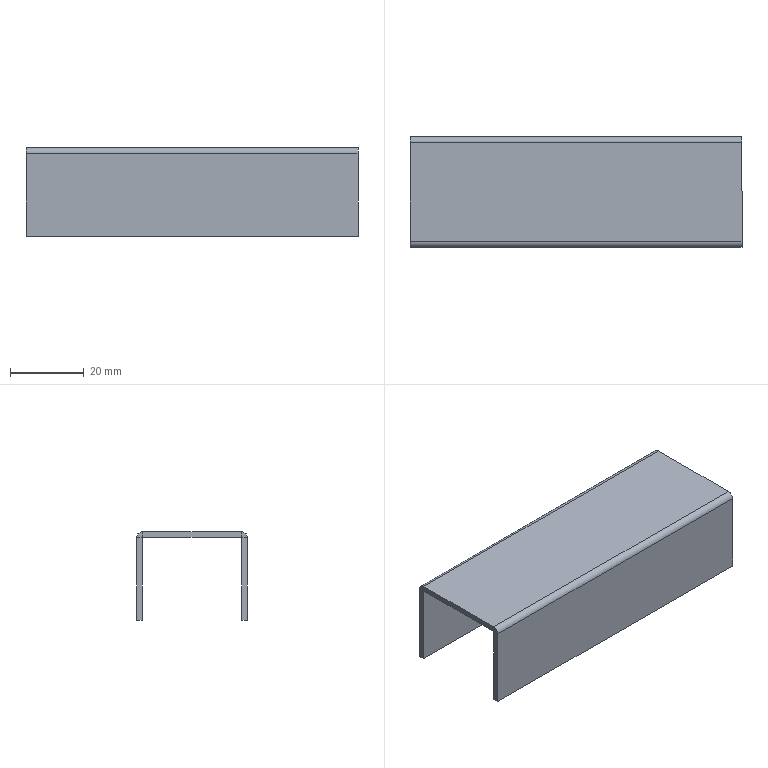Part | SolidWorks | features EdgeFlange 1, FlatPattern 1, SMBaseFlange 1, SheetMetal 1 | 1 solid | 22 faces | box 90 x 30 x 24 mm | volume 10026 mm3 | plane 18 | cylinder 4 | commonest cylinder face diameters 0.2 x2 3.2 x2
STEP:
#1=CARTESIAN_POINT('',(-45.,-13.4,-1.5));
#2=VERTEX_POINT('',#1);
#3=CARTESIAN_POINT('',(45.,-13.4,-1.5));
#4=VERTEX_POINT('',#3);
#5=CARTESIAN_POINT('',(-45.,-13.4,-1.5));
#6=DIRECTION('',(1.,0.,0.));
#7=VECTOR('',#6,1000.);
#8=LINE('',#5,#7);
#9=EDGE_CURVE('',#2,#4,#8,.T.);
#10=ORIENTED_EDGE('',*,*,#9,.F.);
#11=CARTESIAN_POINT('',(-45.,13.4,-1.5));
#12=VERTEX_POINT('',#11);
#13=CARTESIAN_POINT('',(-45.,15.,-1.5));
#14=DIRECTION('',(0.,-1.,0.));
#15=VECTOR('',#14,1000.);
#16=LINE('',#13,#15);
#17=EDGE_CURVE('',#12,#2,#16,.T.);
#18=ORIENTED_EDGE('',*,*,#17,.F.);
#19=CARTESIAN_POINT('',(45.,13.4,-1.5));
#20=VERTEX_POINT('',#19);
#21=CARTESIAN_POINT('',(45.,13.4,-1.5));
#22=DIRECTION('',(-1.,0.,0.));
#23=VECTOR('',#22,1000.);
#24=LINE('',#21,#23);
#25=EDGE_CURVE('',#20,#12,#24,.T.);
#26=ORIENTED_EDGE('',*,*,#25,.F.);
#27=CARTESIAN_POINT('',(45.,15.,-1.5));
#28=DIRECTION('',(0.,1.,0.));
#29=VECTOR('',#28,1000.);
#30=LINE('',#27,#29);
#31=EDGE_CURVE('',#4,#20,#30,.T.);
#32=ORIENTED_EDGE('',*,*,#31,.F.);
#33=EDGE_LOOP('',(#10,#18,#26,#32));
#34=FACE_OUTER_BOUND('',#33,.T.);
#35=CARTESIAN_POINT('',(0.,0.,-1.5));
#36=DIRECTION('',(0.,0.,1.));
#37=DIRECTION('',(1.,0.,0.));
#38=AXIS2_PLACEMENT_3D('',#35,#36,#37);
#39=PLANE('',#38);
#40=ADVANCED_FACE('',(#34),#39,.F.);
#41=CARTESIAN_POINT('',(-45.,13.4,0.));
#42=VERTEX_POINT('',#41);
#43=CARTESIAN_POINT('',(-45.,-13.4,0.));
#44=VERTEX_POINT('',#43);
#45=CARTESIAN_POINT('',(-45.,15.,0.));
#46=DIRECTION('',(0.,-1.,0.));
#47=VECTOR('',#46,1000.);
#48=LINE('',#45,#47);
#49=EDGE_CURVE('',#42,#44,#48,.T.);
#50=ORIENTED_EDGE('',*,*,#49,.T.);
#51=CARTESIAN_POINT('',(45.,-13.4,0.));
#52=VERTEX_POINT('',#51);
#53=CARTESIAN_POINT('',(-45.,-13.4,0.));
#54=DIRECTION('',(1.,0.,0.));
#55=VECTOR('',#54,1000.);
#56=LINE('',#53,#55);
#57=EDGE_CURVE('',#44,#52,#56,.T.);
#58=ORIENTED_EDGE('',*,*,#57,.T.);
#59=CARTESIAN_POINT('',(45.,13.4,0.));
#60=VERTEX_POINT('',#59);
#61=CARTESIAN_POINT('',(45.,15.,0.));
#62=DIRECTION('',(0.,1.,0.));
#63=VECTOR('',#62,1000.);
#64=LINE('',#61,#63);
#65=EDGE_CURVE('',#52,#60,#64,.T.);
#66=ORIENTED_EDGE('',*,*,#65,.T.);
#67=CARTESIAN_POINT('',(45.,13.4,0.));
#68=DIRECTION('',(-1.,0.,0.));
#69=VECTOR('',#68,1000.);
#70=LINE('',#67,#69);
#71=EDGE_CURVE('',#60,#42,#70,.T.);
#72=ORIENTED_EDGE('',*,*,#71,.T.);
#73=EDGE_LOOP('',(#50,#58,#66,#72));
#74=FACE_OUTER_BOUND('',#73,.T.);
#75=CARTESIAN_POINT('',(0.,0.,0.));
#76=DIRECTION('',(0.,0.,1.));
#77=DIRECTION('',(1.,0.,0.));
#78=AXIS2_PLACEMENT_3D('',#75,#76,#77);
#79=PLANE('',#78);
#80=ADVANCED_FACE('',(#74),#79,.T.);
#81=ORIENTED_EDGE('',*,*,#17,.T.);
#82=CARTESIAN_POINT('',(-45.,-13.4,-1.5));
#83=DIRECTION('',(0.,0.,1.));
#84=VECTOR('',#83,1000.);
#85=LINE('',#82,#84);
#86=EDGE_CURVE('',#2,#44,#85,.T.);
#87=ORIENTED_EDGE('',*,*,#86,.T.);
#88=ORIENTED_EDGE('',*,*,#49,.F.);
#89=CARTESIAN_POINT('',(-45.,13.4,-1.5));
#90=DIRECTION('',(0.,0.,1.));
#91=VECTOR('',#90,1000.);
#92=LINE('',#89,#91);
#93=EDGE_CURVE('',#12,#42,#92,.T.);
#94=ORIENTED_EDGE('',*,*,#93,.F.);
#95=EDGE_LOOP('',(#81,#87,#88,#94));
#96=FACE_OUTER_BOUND('',#95,.T.);
#97=CARTESIAN_POINT('',(-45.,15.,-1.5));
#98=DIRECTION('',(-1.,0.,0.));
#99=DIRECTION('',(0.,-1.,0.));
#100=AXIS2_PLACEMENT_3D('',#97,#98,#99);
#101=PLANE('',#100);
#102=ADVANCED_FACE('',(#96),#101,.T.);
#103=CARTESIAN_POINT('',(45.,-13.4,-1.5));
#104=DIRECTION('',(0.,0.,1.));
#105=VECTOR('',#104,1000.);
#106=LINE('',#103,#105);
#107=EDGE_CURVE('',#4,#52,#106,.T.);
#108=ORIENTED_EDGE('',*,*,#107,.F.);
#109=ORIENTED_EDGE('',*,*,#31,.T.);
#110=CARTESIAN_POINT('',(45.,13.4,-1.5));
#111=DIRECTION('',(0.,0.,1.));
#112=VECTOR('',#111,1000.);
#113=LINE('',#110,#112);
#114=EDGE_CURVE('',#20,#60,#113,.T.);
#115=ORIENTED_EDGE('',*,*,#114,.T.);
#116=ORIENTED_EDGE('',*,*,#65,.F.);
#117=EDGE_LOOP('',(#108,#109,#115,#116));
#118=FACE_OUTER_BOUND('',#117,.T.);
#119=CARTESIAN_POINT('',(45.,15.,-1.5));
#120=DIRECTION('',(1.,0.,0.));
#121=DIRECTION('',(0.,1.,0.));
#122=AXIS2_PLACEMENT_3D('',#119,#120,#121);
#123=PLANE('',#122);
#124=ADVANCED_FACE('',(#118),#123,.T.);
#125=CARTESIAN_POINT('',(-45.,13.5,-1.6));
#126=VERTEX_POINT('',#125);
#127=CARTESIAN_POINT('',(-45.,15.,-1.6));
#128=VERTEX_POINT('',#127);
#129=CARTESIAN_POINT('',(-45.,15.,-1.6));
#130=DIRECTION('',(0.,1.,0.));
#131=VECTOR('',#130,1000.);
#132=LINE('',#129,#131);
#133=EDGE_CURVE('',#126,#128,#132,.T.);
#134=ORIENTED_EDGE('',*,*,#133,.F.);
#135=CARTESIAN_POINT('',(-45.,13.4,-1.6));
#136=DIRECTION('',(-1.,0.,0.));
#137=DIRECTION('',(0.,0.,-1.));
#138=AXIS2_PLACEMENT_3D('',#135,#136,#137);
#139=CIRCLE('',#138,0.1);
#140=EDGE_CURVE('',#12,#126,#139,.T.);
#141=ORIENTED_EDGE('',*,*,#140,.F.);
#142=ORIENTED_EDGE('',*,*,#93,.T.);
#143=CARTESIAN_POINT('',(-45.,13.4,-1.6));
#144=DIRECTION('',(-1.,0.,0.));
#145=DIRECTION('',(0.,0.,-1.));
#146=AXIS2_PLACEMENT_3D('',#143,#144,#145);
#147=CIRCLE('',#146,1.6);
#148=EDGE_CURVE('',#42,#128,#147,.T.);
#149=ORIENTED_EDGE('',*,*,#148,.T.);
#150=EDGE_LOOP('',(#134,#141,#142,#149));
#151=FACE_OUTER_BOUND('',#150,.T.);
#152=CARTESIAN_POINT('',(-45.,13.4,-1.6));
#153=DIRECTION('',(-1.,0.,0.));
#154=DIRECTION('',(0.,0.,1.));
#155=AXIS2_PLACEMENT_3D('',#152,#153,#154);
#156=PLANE('',#155);
#157=ADVANCED_FACE('',(#151),#156,.T.);
#158=CARTESIAN_POINT('',(45.,13.5,-1.6));
#159=VERTEX_POINT('',#158);
#160=CARTESIAN_POINT('',(45.,13.4,-1.6));
#161=DIRECTION('',(1.,0.,0.));
#162=DIRECTION('',(0.,0.,-1.));
#163=AXIS2_PLACEMENT_3D('',#160,#161,#162);
#164=CIRCLE('',#163,0.1);
#165=EDGE_CURVE('',#159,#20,#164,.T.);
#166=ORIENTED_EDGE('',*,*,#165,.F.);
#167=CARTESIAN_POINT('',(45.,15.,-1.6));
#168=VERTEX_POINT('',#167);
#169=CARTESIAN_POINT('',(45.,13.5,-1.6));
#170=DIRECTION('',(0.,1.,0.));
#171=VECTOR('',#170,1000.);
#172=LINE('',#169,#171);
#173=EDGE_CURVE('',#159,#168,#172,.T.);
#174=ORIENTED_EDGE('',*,*,#173,.T.);
#175=CARTESIAN_POINT('',(45.,13.4,-1.6));
#176=DIRECTION('',(1.,0.,0.));
#177=DIRECTION('',(0.,0.,-1.));
#178=AXIS2_PLACEMENT_3D('',#175,#176,#177);
#179=CIRCLE('',#178,1.6);
#180=EDGE_CURVE('',#168,#60,#179,.T.);
#181=ORIENTED_EDGE('',*,*,#180,.T.);
#182=ORIENTED_EDGE('',*,*,#114,.F.);
#183=EDGE_LOOP('',(#166,#174,#181,#182));
#184=FACE_OUTER_BOUND('',#183,.T.);
#185=CARTESIAN_POINT('',(45.,13.4,-1.6));
#186=DIRECTION('',(-1.,0.,0.));
#187=DIRECTION('',(0.,0.,1.));
#188=AXIS2_PLACEMENT_3D('',#185,#186,#187);
#189=PLANE('',#188);
#190=ADVANCED_FACE('',(#184),#189,.F.);
#191=ORIENTED_EDGE('',*,*,#71,.F.);
#192=ORIENTED_EDGE('',*,*,#180,.F.);
#193=CARTESIAN_POINT('',(0.,15.,-1.6));
#194=DIRECTION('',(1.,0.,0.));
#195=VECTOR('',#194,1000.);
#196=LINE('',#193,#195);
#197=EDGE_CURVE('',#128,#168,#196,.T.);
#198=ORIENTED_EDGE('',*,*,#197,.F.);
#199=ORIENTED_EDGE('',*,*,#148,.F.);
#200=EDGE_LOOP('',(#191,#192,#198,#199));
#201=FACE_OUTER_BOUND('',#200,.T.);
#202=CARTESIAN_POINT('',(45.,13.4,-1.6));
#203=DIRECTION('',(1.,0.,0.));
#204=DIRECTION('',(0.,1.,0.));
#205=AXIS2_PLACEMENT_3D('',#202,#203,#204);
#206=CYLINDRICAL_SURFACE('',#205,1.6);
#207=ADVANCED_FACE('',(#201),#206,.T.);
#208=ORIENTED_EDGE('',*,*,#25,.T.);
#209=ORIENTED_EDGE('',*,*,#140,.T.);
#210=CARTESIAN_POINT('',(-45.,13.5,-1.6));
#211=DIRECTION('',(1.,0.,0.));
#212=VECTOR('',#211,1000.);
#213=LINE('',#210,#212);
#214=EDGE_CURVE('',#126,#159,#213,.T.);
#215=ORIENTED_EDGE('',*,*,#214,.T.);
#216=ORIENTED_EDGE('',*,*,#165,.T.);
#217=EDGE_LOOP('',(#208,#209,#215,#216));
#218=FACE_OUTER_BOUND('',#217,.T.);
#219=CARTESIAN_POINT('',(45.,13.4,-1.6));
#220=DIRECTION('',(1.,0.,0.));
#221=DIRECTION('',(0.,1.,0.));
#222=AXIS2_PLACEMENT_3D('',#219,#220,#221);
#223=CYLINDRICAL_SURFACE('',#222,0.1);
#224=ADVANCED_FACE('',(#218),#223,.F.);
#225=CARTESIAN_POINT('',(45.,15.,-24.));
#226=VERTEX_POINT('',#225);
#227=CARTESIAN_POINT('',(45.,15.,-1.5));
#228=DIRECTION('',(0.,0.,1.));
#229=VECTOR('',#228,1000.);
#230=LINE('',#227,#229);
#231=EDGE_CURVE('',#226,#168,#230,.T.);
#232=ORIENTED_EDGE('',*,*,#231,.T.);
#233=ORIENTED_EDGE('',*,*,#173,.F.);
#234=CARTESIAN_POINT('',(45.,13.5,-24.));
#235=VERTEX_POINT('',#234);
#236=CARTESIAN_POINT('',(45.,13.5,0.));
#237=DIRECTION('',(0.,0.,1.));
#238=VECTOR('',#237,1000.);
#239=LINE('',#236,#238);
#240=EDGE_CURVE('',#235,#159,#239,.T.);
#241=ORIENTED_EDGE('',*,*,#240,.F.);
#242=CARTESIAN_POINT('',(45.,15.,-24.));
#243=DIRECTION('',(0.,-1.,0.));
#244=VECTOR('',#243,1000.);
#245=LINE('',#242,#244);
#246=EDGE_CURVE('',#226,#235,#245,.T.);
#247=ORIENTED_EDGE('',*,*,#246,.F.);
#248=EDGE_LOOP('',(#232,#233,#241,#247));
#249=FACE_OUTER_BOUND('',#248,.T.);
#250=CARTESIAN_POINT('',(45.,15.,-1.5));
#251=DIRECTION('',(1.,0.,0.));
#252=DIRECTION('',(0.,0.,-1.));
#253=AXIS2_PLACEMENT_3D('',#250,#251,#252);
#254=PLANE('',#253);
#255=ADVANCED_FACE('',(#249),#254,.T.);
#256=CARTESIAN_POINT('',(-45.,13.5,-24.));
#257=VERTEX_POINT('',#256);
#258=CARTESIAN_POINT('',(-45.,13.5,0.));
#259=DIRECTION('',(0.,0.,-1.));
#260=VECTOR('',#259,1000.);
#261=LINE('',#258,#260);
#262=EDGE_CURVE('',#126,#257,#261,.T.);
#263=ORIENTED_EDGE('',*,*,#262,.F.);
#264=ORIENTED_EDGE('',*,*,#133,.T.);
#265=CARTESIAN_POINT('',(-45.,15.,-24.));
#266=VERTEX_POINT('',#265);
#267=CARTESIAN_POINT('',(-45.,15.,-24.));
#268=DIRECTION('',(0.,0.,-1.));
#269=VECTOR('',#268,1000.);
#270=LINE('',#267,#269);
#271=EDGE_CURVE('',#128,#266,#270,.T.);
#272=ORIENTED_EDGE('',*,*,#271,.T.);
#273=CARTESIAN_POINT('',(-45.,15.,-24.));
#274=DIRECTION('',(0.,-1.,0.));
#275=VECTOR('',#274,1000.);
#276=LINE('',#273,#275);
#277=EDGE_CURVE('',#266,#257,#276,.T.);
#278=ORIENTED_EDGE('',*,*,#277,.T.);
#279=EDGE_LOOP('',(#263,#264,#272,#278));
#280=FACE_OUTER_BOUND('',#279,.T.);
#281=CARTESIAN_POINT('',(-45.,15.,-24.));
#282=DIRECTION('',(-1.,0.,0.));
#283=DIRECTION('',(0.,0.,1.));
#284=AXIS2_PLACEMENT_3D('',#281,#282,#283);
#285=PLANE('',#284);
#286=ADVANCED_FACE('',(#280),#285,.T.);
#287=ORIENTED_EDGE('',*,*,#271,.F.);
#288=ORIENTED_EDGE('',*,*,#197,.T.);
#289=ORIENTED_EDGE('',*,*,#231,.F.);
#290=CARTESIAN_POINT('',(45.,15.,-24.));
#291=DIRECTION('',(1.,0.,0.));
#292=VECTOR('',#291,1000.);
#293=LINE('',#290,#292);
#294=EDGE_CURVE('',#266,#226,#293,.T.);
#295=ORIENTED_EDGE('',*,*,#294,.F.);
#296=EDGE_LOOP('',(#287,#288,#289,#295));
#297=FACE_OUTER_BOUND('',#296,.T.);
#298=CARTESIAN_POINT('',(0.,15.,0.));
#299=DIRECTION('',(0.,1.,0.));
#300=DIRECTION('',(0.,0.,1.));
#301=AXIS2_PLACEMENT_3D('',#298,#299,#300);
#302=PLANE('',#301);
#303=ADVANCED_FACE('',(#297),#302,.T.);
#304=ORIENTED_EDGE('',*,*,#214,.F.);
#305=ORIENTED_EDGE('',*,*,#262,.T.);
#306=CARTESIAN_POINT('',(0.,13.5,-24.));
#307=DIRECTION('',(1.,0.,0.));
#308=VECTOR('',#307,1000.);
#309=LINE('',#306,#308);
#310=EDGE_CURVE('',#257,#235,#309,.T.);
#311=ORIENTED_EDGE('',*,*,#310,.T.);
#312=ORIENTED_EDGE('',*,*,#240,.T.);
#313=EDGE_LOOP('',(#304,#305,#311,#312));
#314=FACE_OUTER_BOUND('',#313,.T.);
#315=CARTESIAN_POINT('',(0.,13.5,0.));
#316=DIRECTION('',(0.,1.,0.));
#317=DIRECTION('',(0.,0.,1.));
#318=AXIS2_PLACEMENT_3D('',#315,#316,#317);
#319=PLANE('',#318);
#320=ADVANCED_FACE('',(#314),#319,.F.);
#321=ORIENTED_EDGE('',*,*,#310,.F.);
#322=ORIENTED_EDGE('',*,*,#277,.F.);
#323=ORIENTED_EDGE('',*,*,#294,.T.);
#324=ORIENTED_EDGE('',*,*,#246,.T.);
#325=EDGE_LOOP('',(#321,#322,#323,#324));
#326=FACE_OUTER_BOUND('',#325,.T.);
#327=CARTESIAN_POINT('',(45.,15.,-24.));
#328=DIRECTION('',(0.,0.,-1.));
#329=DIRECTION('',(0.,1.,0.));
#330=AXIS2_PLACEMENT_3D('',#327,#328,#329);
#331=PLANE('',#330);
#332=ADVANCED_FACE('',(#326),#331,.T.);
#333=CARTESIAN_POINT('',(45.,-13.5,-1.6));
#334=VERTEX_POINT('',#333);
#335=CARTESIAN_POINT('',(45.,-15.,-1.6));
#336=VERTEX_POINT('',#335);
#337=CARTESIAN_POINT('',(45.,-15.,-1.6));
#338=DIRECTION('',(0.,-1.,0.));
#339=VECTOR('',#338,1000.);
#340=LINE('',#337,#339);
#341=EDGE_CURVE('',#334,#336,#340,.T.);
#342=ORIENTED_EDGE('',*,*,#341,.F.);
#343=CARTESIAN_POINT('',(45.,-13.4,-1.6));
#344=DIRECTION('',(1.,0.,0.));
#345=DIRECTION('',(0.,0.,1.));
#346=AXIS2_PLACEMENT_3D('',#343,#344,#345);
#347=CIRCLE('',#346,0.1);
#348=EDGE_CURVE('',#4,#334,#347,.T.);
#349=ORIENTED_EDGE('',*,*,#348,.F.);
#350=ORIENTED_EDGE('',*,*,#107,.T.);
#351=CARTESIAN_POINT('',(45.,-13.4,-1.6));
#352=DIRECTION('',(1.,0.,0.));
#353=DIRECTION('',(0.,0.,1.));
#354=AXIS2_PLACEMENT_3D('',#351,#352,#353);
#355=CIRCLE('',#354,1.6);
#356=EDGE_CURVE('',#52,#336,#355,.T.);
#357=ORIENTED_EDGE('',*,*,#356,.T.);
#358=EDGE_LOOP('',(#342,#349,#350,#357));
#359=FACE_OUTER_BOUND('',#358,.T.);
#360=CARTESIAN_POINT('',(45.,-13.4,-1.6));
#361=DIRECTION('',(1.,0.,0.));
#362=DIRECTION('',(0.,0.,-1.));
#363=AXIS2_PLACEMENT_3D('',#360,#361,#362);
#364=PLANE('',#363);
#365=ADVANCED_FACE('',(#359),#364,.T.);
#366=CARTESIAN_POINT('',(-45.,-13.5,-1.6));
#367=VERTEX_POINT('',#366);
#368=CARTESIAN_POINT('',(-45.,-13.4,-1.6));
#369=DIRECTION('',(-1.,0.,0.));
#370=DIRECTION('',(0.,0.,1.));
#371=AXIS2_PLACEMENT_3D('',#368,#369,#370);
#372=CIRCLE('',#371,0.1);
#373=EDGE_CURVE('',#367,#2,#372,.T.);
#374=ORIENTED_EDGE('',*,*,#373,.F.);
#375=CARTESIAN_POINT('',(-45.,-15.,-1.6));
#376=VERTEX_POINT('',#375);
#377=CARTESIAN_POINT('',(-45.,-13.5,-1.6));
#378=DIRECTION('',(0.,-1.,0.));
#379=VECTOR('',#378,1000.);
#380=LINE('',#377,#379);
#381=EDGE_CURVE('',#367,#376,#380,.T.);
#382=ORIENTED_EDGE('',*,*,#381,.T.);
#383=CARTESIAN_POINT('',(-45.,-13.4,-1.6));
#384=DIRECTION('',(-1.,0.,0.));
#385=DIRECTION('',(0.,0.,1.));
#386=AXIS2_PLACEMENT_3D('',#383,#384,#385);
#387=CIRCLE('',#386,1.6);
#388=EDGE_CURVE('',#376,#44,#387,.T.);
#389=ORIENTED_EDGE('',*,*,#388,.T.);
#390=ORIENTED_EDGE('',*,*,#86,.F.);
#391=EDGE_LOOP('',(#374,#382,#389,#390));
#392=FACE_OUTER_BOUND('',#391,.T.);
#393=CARTESIAN_POINT('',(-45.,-13.4,-1.6));
#394=DIRECTION('',(1.,0.,0.));
#395=DIRECTION('',(0.,0.,-1.));
#396=AXIS2_PLACEMENT_3D('',#393,#394,#395);
#397=PLANE('',#396);
#398=ADVANCED_FACE('',(#392),#397,.F.);
#399=ORIENTED_EDGE('',*,*,#57,.F.);
#400=ORIENTED_EDGE('',*,*,#388,.F.);
#401=CARTESIAN_POINT('',(45.,-15.,-1.6));
#402=DIRECTION('',(1.,0.,0.));
#403=VECTOR('',#402,1000.);
#404=LINE('',#401,#403);
#405=EDGE_CURVE('',#376,#336,#404,.T.);
#406=ORIENTED_EDGE('',*,*,#405,.T.);
#407=ORIENTED_EDGE('',*,*,#356,.F.);
#408=EDGE_LOOP('',(#399,#400,#406,#407));
#409=FACE_OUTER_BOUND('',#408,.T.);
#410=CARTESIAN_POINT('',(-45.,-13.4,-1.6));
#411=DIRECTION('',(-1.,0.,0.));
#412=DIRECTION('',(0.,-1.,0.));
#413=AXIS2_PLACEMENT_3D('',#410,#411,#412);
#414=CYLINDRICAL_SURFACE('',#413,1.6);
#415=ADVANCED_FACE('',(#409),#414,.T.);
#416=ORIENTED_EDGE('',*,*,#9,.T.);
#417=ORIENTED_EDGE('',*,*,#348,.T.);
#418=CARTESIAN_POINT('',(45.,-13.5,-1.6));
#419=DIRECTION('',(-1.,0.,0.));
#420=VECTOR('',#419,1000.);
#421=LINE('',#418,#420);
#422=EDGE_CURVE('',#334,#367,#421,.T.);
#423=ORIENTED_EDGE('',*,*,#422,.T.);
#424=ORIENTED_EDGE('',*,*,#373,.T.);
#425=EDGE_LOOP('',(#416,#417,#423,#424));
#426=FACE_OUTER_BOUND('',#425,.T.);
#427=CARTESIAN_POINT('',(-45.,-13.4,-1.6));
#428=DIRECTION('',(-1.,0.,0.));
#429=DIRECTION('',(0.,-1.,0.));
#430=AXIS2_PLACEMENT_3D('',#427,#428,#429);
#431=CYLINDRICAL_SURFACE('',#430,0.1);
#432=ADVANCED_FACE('',(#426),#431,.F.);
#433=CARTESIAN_POINT('',(45.,-13.5,-24.));
#434=VERTEX_POINT('',#433);
#435=CARTESIAN_POINT('',(45.,-13.5,0.));
#436=DIRECTION('',(0.,0.,-1.));
#437=VECTOR('',#436,1000.);
#438=LINE('',#435,#437);
#439=EDGE_CURVE('',#334,#434,#438,.T.);
#440=ORIENTED_EDGE('',*,*,#439,.F.);
#441=ORIENTED_EDGE('',*,*,#341,.T.);
#442=CARTESIAN_POINT('',(45.,-15.,-24.));
#443=VERTEX_POINT('',#442);
#444=CARTESIAN_POINT('',(45.,-15.,-1.5));
#445=DIRECTION('',(0.,0.,-1.));
#446=VECTOR('',#445,1000.);
#447=LINE('',#444,#446);
#448=EDGE_CURVE('',#336,#443,#447,.T.);
#449=ORIENTED_EDGE('',*,*,#448,.T.);
#450=CARTESIAN_POINT('',(45.,-15.,-24.));
#451=DIRECTION('',(0.,1.,0.));
#452=VECTOR('',#451,1000.);
#453=LINE('',#450,#452);
#454=EDGE_CURVE('',#443,#434,#453,.T.);
#455=ORIENTED_EDGE('',*,*,#454,.T.);
#456=EDGE_LOOP('',(#440,#441,#449,#455));
#457=FACE_OUTER_BOUND('',#456,.T.);
#458=CARTESIAN_POINT('',(45.,-15.,-1.5));
#459=DIRECTION('',(1.,0.,0.));
#460=DIRECTION('',(0.,0.,-1.));
#461=AXIS2_PLACEMENT_3D('',#458,#459,#460);
#462=PLANE('',#461);
#463=ADVANCED_FACE('',(#457),#462,.T.);
#464=CARTESIAN_POINT('',(-45.,-15.,-24.));
#465=VERTEX_POINT('',#464);
#466=CARTESIAN_POINT('',(-45.,-15.,-24.));
#467=DIRECTION('',(0.,0.,1.));
#468=VECTOR('',#467,1000.);
#469=LINE('',#466,#468);
#470=EDGE_CURVE('',#465,#376,#469,.T.);
#471=ORIENTED_EDGE('',*,*,#470,.T.);
#472=ORIENTED_EDGE('',*,*,#381,.F.);
#473=CARTESIAN_POINT('',(-45.,-13.5,-24.));
#474=VERTEX_POINT('',#473);
#475=CARTESIAN_POINT('',(-45.,-13.5,0.));
#476=DIRECTION('',(0.,0.,1.));
#477=VECTOR('',#476,1000.);
#478=LINE('',#475,#477);
#479=EDGE_CURVE('',#474,#367,#478,.T.);
#480=ORIENTED_EDGE('',*,*,#479,.F.);
#481=CARTESIAN_POINT('',(-45.,-15.,-24.));
#482=DIRECTION('',(0.,1.,0.));
#483=VECTOR('',#482,1000.);
#484=LINE('',#481,#483);
#485=EDGE_CURVE('',#465,#474,#484,.T.);
#486=ORIENTED_EDGE('',*,*,#485,.F.);
#487=EDGE_LOOP('',(#471,#472,#480,#486));
#488=FACE_OUTER_BOUND('',#487,.T.);
#489=CARTESIAN_POINT('',(-45.,-15.,-24.));
#490=DIRECTION('',(-1.,0.,0.));
#491=DIRECTION('',(0.,0.,1.));
#492=AXIS2_PLACEMENT_3D('',#489,#490,#491);
#493=PLANE('',#492);
#494=ADVANCED_FACE('',(#488),#493,.T.);
#495=ORIENTED_EDGE('',*,*,#405,.F.);
#496=ORIENTED_EDGE('',*,*,#470,.F.);
#497=CARTESIAN_POINT('',(45.,-15.,-24.));
#498=DIRECTION('',(-1.,0.,0.));
#499=VECTOR('',#498,1000.);
#500=LINE('',#497,#499);
#501=EDGE_CURVE('',#443,#465,#500,.T.);
#502=ORIENTED_EDGE('',*,*,#501,.F.);
#503=ORIENTED_EDGE('',*,*,#448,.F.);
#504=EDGE_LOOP('',(#495,#496,#502,#503));
#505=FACE_OUTER_BOUND('',#504,.T.);
#506=CARTESIAN_POINT('',(0.,-15.,0.));
#507=DIRECTION('',(0.,1.,0.));
#508=DIRECTION('',(0.,0.,1.));
#509=AXIS2_PLACEMENT_3D('',#506,#507,#508);
#510=PLANE('',#509);
#511=ADVANCED_FACE('',(#505),#510,.F.);
#512=ORIENTED_EDGE('',*,*,#479,.T.);
#513=ORIENTED_EDGE('',*,*,#422,.F.);
#514=ORIENTED_EDGE('',*,*,#439,.T.);
#515=CARTESIAN_POINT('',(0.,-13.5,-24.));
#516=DIRECTION('',(-1.,0.,0.));
#517=VECTOR('',#516,1000.);
#518=LINE('',#515,#517);
#519=EDGE_CURVE('',#434,#474,#518,.T.);
#520=ORIENTED_EDGE('',*,*,#519,.T.);
#521=EDGE_LOOP('',(#512,#513,#514,#520));
#522=FACE_OUTER_BOUND('',#521,.T.);
#523=CARTESIAN_POINT('',(0.,-13.5,0.));
#524=DIRECTION('',(0.,1.,0.));
#525=DIRECTION('',(0.,0.,1.));
#526=AXIS2_PLACEMENT_3D('',#523,#524,#525);
#527=PLANE('',#526);
#528=ADVANCED_FACE('',(#522),#527,.T.);
#529=ORIENTED_EDGE('',*,*,#519,.F.);
#530=ORIENTED_EDGE('',*,*,#454,.F.);
#531=ORIENTED_EDGE('',*,*,#501,.T.);
#532=ORIENTED_EDGE('',*,*,#485,.T.);
#533=EDGE_LOOP('',(#529,#530,#531,#532));
#534=FACE_OUTER_BOUND('',#533,.T.);
#535=CARTESIAN_POINT('',(45.,-15.,-24.));
#536=DIRECTION('',(0.,0.,-1.));
#537=DIRECTION('',(0.,1.,0.));
#538=AXIS2_PLACEMENT_3D('',#535,#536,#537);
#539=PLANE('',#538);
#540=ADVANCED_FACE('',(#534),#539,.T.);
#541=CLOSED_SHELL('',(#40,#80,#102,#124,#157,#190,#207,#224,#255,#286,#303,#320,#332,#365,#398,#415,#432,#463,#494,#511,#528,#540));
#542=MANIFOLD_SOLID_BREP('',#541);
#543=CARTESIAN_POINT('',(0.,0.,0.));
#544=DIRECTION('',(0.,0.,1.));
#545=DIRECTION('',(1.,0.,0.));
#546=AXIS2_PLACEMENT_3D('',#543,#544,#545);
#547=(LENGTH_UNIT()NAMED_UNIT(*)SI_UNIT(.MILLI.,.METRE.));
#548=UNCERTAINTY_MEASURE_WITH_UNIT(LENGTH_MEASURE(0.00001),#547,'','');
#549=(NAMED_UNIT(*)PLANE_ANGLE_UNIT()SI_UNIT($,.RADIAN.));
#550=(NAMED_UNIT(*)SI_UNIT($,.STERADIAN.)SOLID_ANGLE_UNIT());
#551=(GEOMETRIC_REPRESENTATION_CONTEXT(3)GLOBAL_UNCERTAINTY_ASSIGNED_CONTEXT((#548))GLOBAL_UNIT_ASSIGNED_CONTEXT((#547,#549,#550))REPRESENTATION_CONTEXT('',''));
#552=ADVANCED_BREP_SHAPE_REPRESENTATION('',(#542,#546),#551);